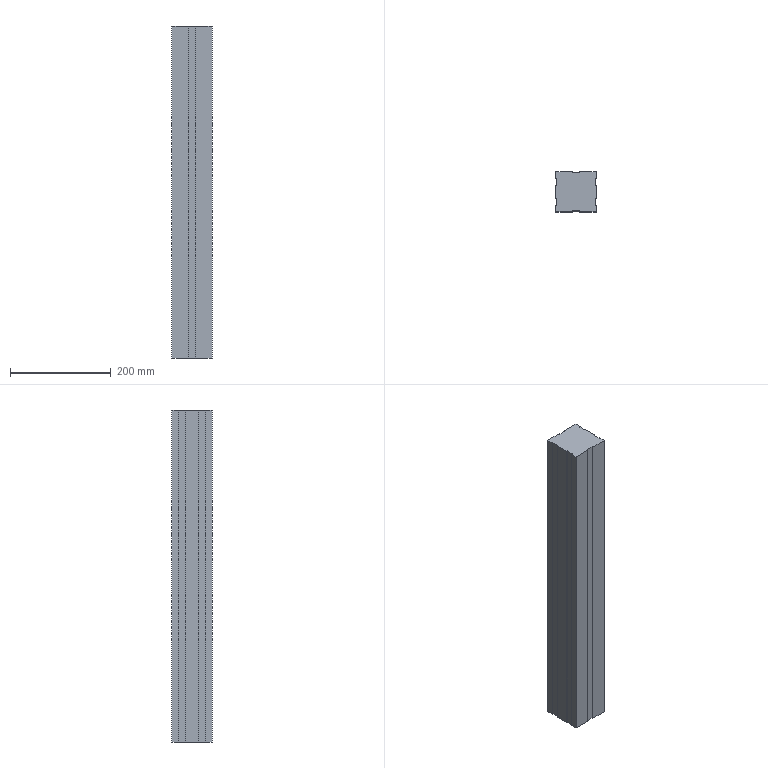Part | STEP file | xingcai80x80x420 | 1 solid | 30 faces | box 80 x 80 x 660 mm | volume 4113120 mm3 | plane 30